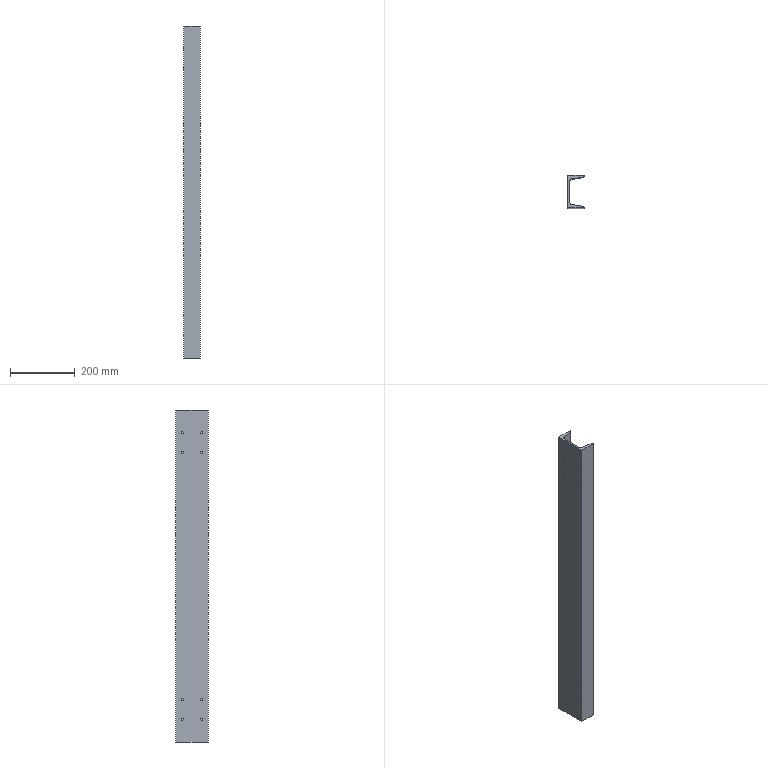Part | SolidWorks | features Extrusion 1, HoleWzd 1 | 1 solid | 30 faces | box 50 x 100 x 1022 mm | volume 1354327 mm3 | cylinder 20 | plane 10 | commonest cylinder face diameters 6.8 x16 9 x2 17 x2
STEP:
#1=CARTESIAN_POINT('',(-44.,-20.,66.6));
#2=VERTEX_POINT('',#1);
#3=CARTESIAN_POINT('',(-44.,-20.,73.4));
#4=VERTEX_POINT('',#3);
#5=CARTESIAN_POINT('',(-44.,-20.,70.));
#6=DIRECTION('',(-1.,0.,0.));
#7=DIRECTION('',(0.,0.,1.));
#8=AXIS2_PLACEMENT_3D('',#5,#6,#7);
#9=CIRCLE('',#8,3.4);
#10=EDGE_CURVE('',#2,#4,#9,.T.);
#11=ORIENTED_EDGE('',*,*,#10,.F.);
#12=CARTESIAN_POINT('',(-50.,-20.,66.6));
#13=VERTEX_POINT('',#12);
#14=CARTESIAN_POINT('',(-50.,-20.,66.6));
#15=DIRECTION('',(-1.,0.,0.));
#16=VECTOR('',#15,1000.);
#17=LINE('',#14,#16);
#18=EDGE_CURVE('',#2,#13,#17,.T.);
#19=ORIENTED_EDGE('',*,*,#18,.T.);
#20=CARTESIAN_POINT('',(-50.,-20.,73.4));
#21=VERTEX_POINT('',#20);
#22=CARTESIAN_POINT('',(-50.,-20.,70.));
#23=DIRECTION('',(-1.,0.,0.));
#24=DIRECTION('',(0.,0.,1.));
#25=AXIS2_PLACEMENT_3D('',#22,#23,#24);
#26=CIRCLE('',#25,3.4);
#27=EDGE_CURVE('',#13,#21,#26,.T.);
#28=ORIENTED_EDGE('',*,*,#27,.T.);
#29=CARTESIAN_POINT('',(-50.,-20.,73.4));
#30=DIRECTION('',(-1.,0.,0.));
#31=VECTOR('',#30,1000.);
#32=LINE('',#29,#31);
#33=EDGE_CURVE('',#4,#21,#32,.T.);
#34=ORIENTED_EDGE('',*,*,#33,.F.);
#35=EDGE_LOOP('',(#11,#19,#28,#34));
#36=FACE_OUTER_BOUND('',#35,.T.);
#37=CARTESIAN_POINT('',(-50.,-20.,70.));
#38=DIRECTION('',(-1.,0.,0.));
#39=DIRECTION('',(0.,0.,1.));
#40=AXIS2_PLACEMENT_3D('',#37,#38,#39);
#41=CYLINDRICAL_SURFACE('',#40,3.4);
#42=ADVANCED_FACE('',(#36),#41,.F.);
#43=CARTESIAN_POINT('',(-44.,-20.,126.6));
#44=VERTEX_POINT('',#43);
#45=CARTESIAN_POINT('',(-44.,-20.,133.4));
#46=VERTEX_POINT('',#45);
#47=CARTESIAN_POINT('',(-44.,-20.,130.));
#48=DIRECTION('',(-1.,0.,0.));
#49=DIRECTION('',(0.,0.,1.));
#50=AXIS2_PLACEMENT_3D('',#47,#48,#49);
#51=CIRCLE('',#50,3.4);
#52=EDGE_CURVE('',#44,#46,#51,.T.);
#53=ORIENTED_EDGE('',*,*,#52,.F.);
#54=CARTESIAN_POINT('',(-50.,-20.,126.6));
#55=VERTEX_POINT('',#54);
#56=CARTESIAN_POINT('',(-50.,-20.,126.6));
#57=DIRECTION('',(-1.,0.,0.));
#58=VECTOR('',#57,1000.);
#59=LINE('',#56,#58);
#60=EDGE_CURVE('',#44,#55,#59,.T.);
#61=ORIENTED_EDGE('',*,*,#60,.T.);
#62=CARTESIAN_POINT('',(-50.,-20.,133.4));
#63=VERTEX_POINT('',#62);
#64=CARTESIAN_POINT('',(-50.,-20.,130.));
#65=DIRECTION('',(-1.,0.,0.));
#66=DIRECTION('',(0.,0.,1.));
#67=AXIS2_PLACEMENT_3D('',#64,#65,#66);
#68=CIRCLE('',#67,3.4);
#69=EDGE_CURVE('',#55,#63,#68,.T.);
#70=ORIENTED_EDGE('',*,*,#69,.T.);
#71=CARTESIAN_POINT('',(-50.,-20.,133.4));
#72=DIRECTION('',(-1.,0.,0.));
#73=VECTOR('',#72,1000.);
#74=LINE('',#71,#73);
#75=EDGE_CURVE('',#46,#63,#74,.T.);
#76=ORIENTED_EDGE('',*,*,#75,.F.);
#77=EDGE_LOOP('',(#53,#61,#70,#76));
#78=FACE_OUTER_BOUND('',#77,.T.);
#79=CARTESIAN_POINT('',(-50.,-20.,130.));
#80=DIRECTION('',(-1.,0.,0.));
#81=DIRECTION('',(0.,0.,1.));
#82=AXIS2_PLACEMENT_3D('',#79,#80,#81);
#83=CYLINDRICAL_SURFACE('',#82,3.4);
#84=ADVANCED_FACE('',(#78),#83,.F.);
#85=CARTESIAN_POINT('',(-44.,-80.,126.6));
#86=VERTEX_POINT('',#85);
#87=CARTESIAN_POINT('',(-44.,-81.441,126.92));
#88=VERTEX_POINT('',#87);
#89=CARTESIAN_POINT('',(-44.,-80.,130.));
#90=DIRECTION('',(-1.,0.,0.));
#91=DIRECTION('',(0.,0.,1.));
#92=AXIS2_PLACEMENT_3D('',#89,#90,#91);
#93=CIRCLE('',#92,3.4);
#94=EDGE_CURVE('',#86,#88,#93,.T.);
#95=ORIENTED_EDGE('',*,*,#94,.F.);
#96=CARTESIAN_POINT('',(-50.,-80.,126.6));
#97=VERTEX_POINT('',#96);
#98=CARTESIAN_POINT('',(-50.,-80.,126.6));
#99=DIRECTION('',(-1.,0.,0.));
#100=VECTOR('',#99,1000.);
#101=LINE('',#98,#100);
#102=EDGE_CURVE('',#86,#97,#101,.T.);
#103=ORIENTED_EDGE('',*,*,#102,.T.);
#104=CARTESIAN_POINT('',(-50.,-80.,133.4));
#105=VERTEX_POINT('',#104);
#106=CARTESIAN_POINT('',(-50.,-80.,130.));
#107=DIRECTION('',(-1.,0.,0.));
#108=DIRECTION('',(0.,0.,1.));
#109=AXIS2_PLACEMENT_3D('',#106,#107,#108);
#110=CIRCLE('',#109,3.4);
#111=EDGE_CURVE('',#97,#105,#110,.T.);
#112=ORIENTED_EDGE('',*,*,#111,.T.);
#113=CARTESIAN_POINT('',(-44.,-80.,133.4));
#114=VERTEX_POINT('',#113);
#115=CARTESIAN_POINT('',(-50.,-80.,133.4));
#116=DIRECTION('',(-1.,0.,0.));
#117=VECTOR('',#116,1000.);
#118=LINE('',#115,#117);
#119=EDGE_CURVE('',#114,#105,#118,.T.);
#120=ORIENTED_EDGE('',*,*,#119,.F.);
#121=CARTESIAN_POINT('',(-44.,-81.441,133.08));
#122=VERTEX_POINT('',#121);
#123=CARTESIAN_POINT('',(-44.,-80.,130.));
#124=DIRECTION('',(-1.,0.,0.));
#125=DIRECTION('',(0.,0.,1.));
#126=AXIS2_PLACEMENT_3D('',#123,#124,#125);
#127=CIRCLE('',#126,3.4);
#128=EDGE_CURVE('',#122,#114,#127,.T.);
#129=ORIENTED_EDGE('',*,*,#128,.F.);
#130=CARTESIAN_POINT('',(-44.,-81.441,126.92));
#131=CARTESIAN_POINT('',(-44.,-81.735,127.058));
#132=CARTESIAN_POINT('',(-43.985,-82.002,127.233));
#133=CARTESIAN_POINT('',(-43.951,-82.365,127.552));
#134=CARTESIAN_POINT('',(-43.937,-82.479,127.667));
#135=CARTESIAN_POINT('',(-43.909,-82.687,127.91));
#136=CARTESIAN_POINT('',(-43.894,-82.782,128.039));
#137=CARTESIAN_POINT('',(-43.865,-82.954,128.308));
#138=CARTESIAN_POINT('',(-43.85,-83.031,128.451));
#139=CARTESIAN_POINT('',(-43.824,-83.163,128.744));
#140=CARTESIAN_POINT('',(-43.812,-83.219,128.894));
#141=CARTESIAN_POINT('',(-43.783,-83.353,129.353));
#142=CARTESIAN_POINT('',(-43.771,-83.4,129.679));
#143=CARTESIAN_POINT('',(-43.771,-83.4,130.159));
#144=CARTESIAN_POINT('',(-43.774,-83.389,130.319));
#145=CARTESIAN_POINT('',(-43.784,-83.344,130.637));
#146=CARTESIAN_POINT('',(-43.792,-83.309,130.796));
#147=CARTESIAN_POINT('',(-43.812,-83.22,131.105));
#148=CARTESIAN_POINT('',(-43.824,-83.164,131.254));
#149=CARTESIAN_POINT('',(-43.85,-83.033,131.546));
#150=CARTESIAN_POINT('',(-43.864,-82.956,131.688));
#151=CARTESIAN_POINT('',(-43.909,-82.697,132.095));
#152=CARTESIAN_POINT('',(-43.939,-82.49,132.338));
#153=CARTESIAN_POINT('',(-43.985,-82.005,132.765));
#154=CARTESIAN_POINT('',(-44.,-81.735,132.942));
#155=CARTESIAN_POINT('',(-44.,-81.441,133.08));
#156=B_SPLINE_CURVE_WITH_KNOTS('',3,(#130,#131,#132,#133,#134,#135,#136,#137,#138,#139,#140,#141,#142,#143,#144,#145,#146,#147,#148,#149,#150,#151,#152,#153,#154,#155),.UNSPECIFIED.,.F.,.F.,(4,2,2,2,2,2,2,2,2,2,2,2,4),(0.,0.0009601,0.00144,0.00192,0.0024,0.00288,0.003841,0.004321,0.004801,0.005281,0.005761,0.006721,0.007681),.UNSPECIFIED.);
#157=EDGE_CURVE('',#88,#122,#156,.T.);
#158=ORIENTED_EDGE('',*,*,#157,.F.);
#159=EDGE_LOOP('',(#95,#103,#112,#120,#129,#158));
#160=FACE_OUTER_BOUND('',#159,.T.);
#161=CARTESIAN_POINT('',(-50.,-80.,130.));
#162=DIRECTION('',(-1.,0.,0.));
#163=DIRECTION('',(0.,0.,1.));
#164=AXIS2_PLACEMENT_3D('',#161,#162,#163);
#165=CYLINDRICAL_SURFACE('',#164,3.4);
#166=ADVANCED_FACE('',(#160),#165,.F.);
#167=CARTESIAN_POINT('',(-44.,-80.,66.6));
#168=VERTEX_POINT('',#167);
#169=CARTESIAN_POINT('',(-44.,-81.441,66.92));
#170=VERTEX_POINT('',#169);
#171=CARTESIAN_POINT('',(-44.,-80.,70.));
#172=DIRECTION('',(-1.,0.,0.));
#173=DIRECTION('',(0.,0.,1.));
#174=AXIS2_PLACEMENT_3D('',#171,#172,#173);
#175=CIRCLE('',#174,3.4);
#176=EDGE_CURVE('',#168,#170,#175,.T.);
#177=ORIENTED_EDGE('',*,*,#176,.F.);
#178=CARTESIAN_POINT('',(-50.,-80.,66.6));
#179=VERTEX_POINT('',#178);
#180=CARTESIAN_POINT('',(-50.,-80.,66.6));
#181=DIRECTION('',(-1.,0.,0.));
#182=VECTOR('',#181,1000.);
#183=LINE('',#180,#182);
#184=EDGE_CURVE('',#168,#179,#183,.T.);
#185=ORIENTED_EDGE('',*,*,#184,.T.);
#186=CARTESIAN_POINT('',(-50.,-80.,73.4));
#187=VERTEX_POINT('',#186);
#188=CARTESIAN_POINT('',(-50.,-80.,70.));
#189=DIRECTION('',(-1.,0.,0.));
#190=DIRECTION('',(0.,0.,1.));
#191=AXIS2_PLACEMENT_3D('',#188,#189,#190);
#192=CIRCLE('',#191,3.4);
#193=EDGE_CURVE('',#179,#187,#192,.T.);
#194=ORIENTED_EDGE('',*,*,#193,.T.);
#195=CARTESIAN_POINT('',(-44.,-80.,73.4));
#196=VERTEX_POINT('',#195);
#197=CARTESIAN_POINT('',(-50.,-80.,73.4));
#198=DIRECTION('',(-1.,0.,0.));
#199=VECTOR('',#198,1000.);
#200=LINE('',#197,#199);
#201=EDGE_CURVE('',#196,#187,#200,.T.);
#202=ORIENTED_EDGE('',*,*,#201,.F.);
#203=CARTESIAN_POINT('',(-44.,-81.441,73.08));
#204=VERTEX_POINT('',#203);
#205=CARTESIAN_POINT('',(-44.,-80.,70.));
#206=DIRECTION('',(-1.,0.,0.));
#207=DIRECTION('',(0.,0.,1.));
#208=AXIS2_PLACEMENT_3D('',#205,#206,#207);
#209=CIRCLE('',#208,3.4);
#210=EDGE_CURVE('',#204,#196,#209,.T.);
#211=ORIENTED_EDGE('',*,*,#210,.F.);
#212=CARTESIAN_POINT('',(-44.,-81.441,66.92));
#213=CARTESIAN_POINT('',(-44.,-81.735,67.058));
#214=CARTESIAN_POINT('',(-43.985,-82.002,67.233));
#215=CARTESIAN_POINT('',(-43.951,-82.365,67.552));
#216=CARTESIAN_POINT('',(-43.937,-82.479,67.667));
#217=CARTESIAN_POINT('',(-43.909,-82.687,67.91));
#218=CARTESIAN_POINT('',(-43.894,-82.782,68.039));
#219=CARTESIAN_POINT('',(-43.865,-82.954,68.308));
#220=CARTESIAN_POINT('',(-43.85,-83.031,68.451));
#221=CARTESIAN_POINT('',(-43.824,-83.163,68.744));
#222=CARTESIAN_POINT('',(-43.812,-83.219,68.894));
#223=CARTESIAN_POINT('',(-43.783,-83.353,69.353));
#224=CARTESIAN_POINT('',(-43.771,-83.4,69.679));
#225=CARTESIAN_POINT('',(-43.771,-83.4,70.159));
#226=CARTESIAN_POINT('',(-43.774,-83.389,70.319));
#227=CARTESIAN_POINT('',(-43.784,-83.344,70.637));
#228=CARTESIAN_POINT('',(-43.792,-83.309,70.796));
#229=CARTESIAN_POINT('',(-43.812,-83.22,71.105));
#230=CARTESIAN_POINT('',(-43.824,-83.164,71.254));
#231=CARTESIAN_POINT('',(-43.85,-83.033,71.546));
#232=CARTESIAN_POINT('',(-43.864,-82.956,71.688));
#233=CARTESIAN_POINT('',(-43.909,-82.697,72.095));
#234=CARTESIAN_POINT('',(-43.939,-82.49,72.338));
#235=CARTESIAN_POINT('',(-43.985,-82.005,72.765));
#236=CARTESIAN_POINT('',(-44.,-81.735,72.942));
#237=CARTESIAN_POINT('',(-44.,-81.441,73.08));
#238=B_SPLINE_CURVE_WITH_KNOTS('',3,(#212,#213,#214,#215,#216,#217,#218,#219,#220,#221,#222,#223,#224,#225,#226,#227,#228,#229,#230,#231,#232,#233,#234,#235,#236,#237),.UNSPECIFIED.,.F.,.F.,(4,2,2,2,2,2,2,2,2,2,2,2,4),(0.,0.0009601,0.00144,0.00192,0.0024,0.00288,0.003841,0.004321,0.004801,0.005281,0.005761,0.006721,0.007681),.UNSPECIFIED.);
#239=EDGE_CURVE('',#170,#204,#238,.T.);
#240=ORIENTED_EDGE('',*,*,#239,.F.);
#241=EDGE_LOOP('',(#177,#185,#194,#202,#211,#240));
#242=FACE_OUTER_BOUND('',#241,.T.);
#243=CARTESIAN_POINT('',(-50.,-80.,70.));
#244=DIRECTION('',(-1.,0.,0.));
#245=DIRECTION('',(0.,0.,1.));
#246=AXIS2_PLACEMENT_3D('',#243,#244,#245);
#247=CYLINDRICAL_SURFACE('',#246,3.4);
#248=ADVANCED_FACE('',(#242),#247,.F.);
#249=CARTESIAN_POINT('',(-44.,-20.,888.6));
#250=VERTEX_POINT('',#249);
#251=CARTESIAN_POINT('',(-44.,-20.,895.4));
#252=VERTEX_POINT('',#251);
#253=CARTESIAN_POINT('',(-44.,-20.,892.));
#254=DIRECTION('',(-1.,0.,0.));
#255=DIRECTION('',(0.,0.,1.));
#256=AXIS2_PLACEMENT_3D('',#253,#254,#255);
#257=CIRCLE('',#256,3.4);
#258=EDGE_CURVE('',#250,#252,#257,.T.);
#259=ORIENTED_EDGE('',*,*,#258,.F.);
#260=CARTESIAN_POINT('',(-50.,-20.,888.6));
#261=VERTEX_POINT('',#260);
#262=CARTESIAN_POINT('',(-50.,-20.,888.6));
#263=DIRECTION('',(-1.,0.,0.));
#264=VECTOR('',#263,1000.);
#265=LINE('',#262,#264);
#266=EDGE_CURVE('',#250,#261,#265,.T.);
#267=ORIENTED_EDGE('',*,*,#266,.T.);
#268=CARTESIAN_POINT('',(-50.,-20.,895.4));
#269=VERTEX_POINT('',#268);
#270=CARTESIAN_POINT('',(-50.,-20.,892.));
#271=DIRECTION('',(-1.,0.,0.));
#272=DIRECTION('',(0.,0.,1.));
#273=AXIS2_PLACEMENT_3D('',#270,#271,#272);
#274=CIRCLE('',#273,3.4);
#275=EDGE_CURVE('',#261,#269,#274,.T.);
#276=ORIENTED_EDGE('',*,*,#275,.T.);
#277=CARTESIAN_POINT('',(-50.,-20.,895.4));
#278=DIRECTION('',(-1.,0.,0.));
#279=VECTOR('',#278,1000.);
#280=LINE('',#277,#279);
#281=EDGE_CURVE('',#252,#269,#280,.T.);
#282=ORIENTED_EDGE('',*,*,#281,.F.);
#283=EDGE_LOOP('',(#259,#267,#276,#282));
#284=FACE_OUTER_BOUND('',#283,.T.);
#285=CARTESIAN_POINT('',(-50.,-20.,892.));
#286=DIRECTION('',(-1.,0.,0.));
#287=DIRECTION('',(0.,0.,1.));
#288=AXIS2_PLACEMENT_3D('',#285,#286,#287);
#289=CYLINDRICAL_SURFACE('',#288,3.4);
#290=ADVANCED_FACE('',(#284),#289,.F.);
#291=CARTESIAN_POINT('',(-44.,-20.,948.6));
#292=VERTEX_POINT('',#291);
#293=CARTESIAN_POINT('',(-44.,-20.,955.4));
#294=VERTEX_POINT('',#293);
#295=CARTESIAN_POINT('',(-44.,-20.,952.));
#296=DIRECTION('',(-1.,0.,0.));
#297=DIRECTION('',(0.,0.,1.));
#298=AXIS2_PLACEMENT_3D('',#295,#296,#297);
#299=CIRCLE('',#298,3.4);
#300=EDGE_CURVE('',#292,#294,#299,.T.);
#301=ORIENTED_EDGE('',*,*,#300,.F.);
#302=CARTESIAN_POINT('',(-50.,-20.,948.6));
#303=VERTEX_POINT('',#302);
#304=CARTESIAN_POINT('',(-50.,-20.,948.6));
#305=DIRECTION('',(-1.,0.,0.));
#306=VECTOR('',#305,1000.);
#307=LINE('',#304,#306);
#308=EDGE_CURVE('',#292,#303,#307,.T.);
#309=ORIENTED_EDGE('',*,*,#308,.T.);
#310=CARTESIAN_POINT('',(-50.,-20.,955.4));
#311=VERTEX_POINT('',#310);
#312=CARTESIAN_POINT('',(-50.,-20.,952.));
#313=DIRECTION('',(-1.,0.,0.));
#314=DIRECTION('',(0.,0.,1.));
#315=AXIS2_PLACEMENT_3D('',#312,#313,#314);
#316=CIRCLE('',#315,3.4);
#317=EDGE_CURVE('',#303,#311,#316,.T.);
#318=ORIENTED_EDGE('',*,*,#317,.T.);
#319=CARTESIAN_POINT('',(-50.,-20.,955.4));
#320=DIRECTION('',(-1.,0.,0.));
#321=VECTOR('',#320,1000.);
#322=LINE('',#319,#321);
#323=EDGE_CURVE('',#294,#311,#322,.T.);
#324=ORIENTED_EDGE('',*,*,#323,.F.);
#325=EDGE_LOOP('',(#301,#309,#318,#324));
#326=FACE_OUTER_BOUND('',#325,.T.);
#327=CARTESIAN_POINT('',(-50.,-20.,952.));
#328=DIRECTION('',(-1.,0.,0.));
#329=DIRECTION('',(0.,0.,1.));
#330=AXIS2_PLACEMENT_3D('',#327,#328,#329);
#331=CYLINDRICAL_SURFACE('',#330,3.4);
#332=ADVANCED_FACE('',(#326),#331,.F.);
#333=CARTESIAN_POINT('',(-44.,-80.,948.6));
#334=VERTEX_POINT('',#333);
#335=CARTESIAN_POINT('',(-44.,-81.441,948.92));
#336=VERTEX_POINT('',#335);
#337=CARTESIAN_POINT('',(-44.,-80.,952.));
#338=DIRECTION('',(-1.,0.,0.));
#339=DIRECTION('',(0.,0.,1.));
#340=AXIS2_PLACEMENT_3D('',#337,#338,#339);
#341=CIRCLE('',#340,3.4);
#342=EDGE_CURVE('',#334,#336,#341,.T.);
#343=ORIENTED_EDGE('',*,*,#342,.F.);
#344=CARTESIAN_POINT('',(-50.,-80.,948.6));
#345=VERTEX_POINT('',#344);
#346=CARTESIAN_POINT('',(-50.,-80.,948.6));
#347=DIRECTION('',(-1.,0.,0.));
#348=VECTOR('',#347,1000.);
#349=LINE('',#346,#348);
#350=EDGE_CURVE('',#334,#345,#349,.T.);
#351=ORIENTED_EDGE('',*,*,#350,.T.);
#352=CARTESIAN_POINT('',(-50.,-80.,955.4));
#353=VERTEX_POINT('',#352);
#354=CARTESIAN_POINT('',(-50.,-80.,952.));
#355=DIRECTION('',(-1.,0.,0.));
#356=DIRECTION('',(0.,0.,1.));
#357=AXIS2_PLACEMENT_3D('',#354,#355,#356);
#358=CIRCLE('',#357,3.4);
#359=EDGE_CURVE('',#345,#353,#358,.T.);
#360=ORIENTED_EDGE('',*,*,#359,.T.);
#361=CARTESIAN_POINT('',(-44.,-80.,955.4));
#362=VERTEX_POINT('',#361);
#363=CARTESIAN_POINT('',(-50.,-80.,955.4));
#364=DIRECTION('',(-1.,0.,0.));
#365=VECTOR('',#364,1000.);
#366=LINE('',#363,#365);
#367=EDGE_CURVE('',#362,#353,#366,.T.);
#368=ORIENTED_EDGE('',*,*,#367,.F.);
#369=CARTESIAN_POINT('',(-44.,-81.441,955.08));
#370=VERTEX_POINT('',#369);
#371=CARTESIAN_POINT('',(-44.,-80.,952.));
#372=DIRECTION('',(-1.,0.,0.));
#373=DIRECTION('',(0.,0.,1.));
#374=AXIS2_PLACEMENT_3D('',#371,#372,#373);
#375=CIRCLE('',#374,3.4);
#376=EDGE_CURVE('',#370,#362,#375,.T.);
#377=ORIENTED_EDGE('',*,*,#376,.F.);
#378=CARTESIAN_POINT('',(-44.,-81.441,948.92));
#379=CARTESIAN_POINT('',(-44.,-81.735,949.058));
#380=CARTESIAN_POINT('',(-43.985,-82.002,949.233));
#381=CARTESIAN_POINT('',(-43.951,-82.365,949.552));
#382=CARTESIAN_POINT('',(-43.937,-82.479,949.667));
#383=CARTESIAN_POINT('',(-43.909,-82.687,949.91));
#384=CARTESIAN_POINT('',(-43.894,-82.782,950.039));
#385=CARTESIAN_POINT('',(-43.865,-82.954,950.308));
#386=CARTESIAN_POINT('',(-43.85,-83.031,950.451));
#387=CARTESIAN_POINT('',(-43.824,-83.163,950.744));
#388=CARTESIAN_POINT('',(-43.812,-83.219,950.894));
#389=CARTESIAN_POINT('',(-43.783,-83.353,951.353));
#390=CARTESIAN_POINT('',(-43.771,-83.4,951.679));
#391=CARTESIAN_POINT('',(-43.771,-83.4,952.159));
#392=CARTESIAN_POINT('',(-43.774,-83.389,952.319));
#393=CARTESIAN_POINT('',(-43.784,-83.344,952.637));
#394=CARTESIAN_POINT('',(-43.792,-83.309,952.796));
#395=CARTESIAN_POINT('',(-43.812,-83.22,953.105));
#396=CARTESIAN_POINT('',(-43.824,-83.164,953.254));
#397=CARTESIAN_POINT('',(-43.85,-83.033,953.546));
#398=CARTESIAN_POINT('',(-43.864,-82.956,953.688));
#399=CARTESIAN_POINT('',(-43.909,-82.697,954.095));
#400=CARTESIAN_POINT('',(-43.939,-82.49,954.338));
#401=CARTESIAN_POINT('',(-43.985,-82.005,954.765));
#402=CARTESIAN_POINT('',(-44.,-81.735,954.942));
#403=CARTESIAN_POINT('',(-44.,-81.441,955.08));
#404=B_SPLINE_CURVE_WITH_KNOTS('',3,(#378,#379,#380,#381,#382,#383,#384,#385,#386,#387,#388,#389,#390,#391,#392,#393,#394,#395,#396,#397,#398,#399,#400,#401,#402,#403),.UNSPECIFIED.,.F.,.F.,(4,2,2,2,2,2,2,2,2,2,2,2,4),(0.,0.0009601,0.00144,0.00192,0.0024,0.00288,0.003841,0.004321,0.004801,0.005281,0.005761,0.006721,0.007681),.UNSPECIFIED.);
#405=EDGE_CURVE('',#336,#370,#404,.T.);
#406=ORIENTED_EDGE('',*,*,#405,.F.);
#407=EDGE_LOOP('',(#343,#351,#360,#368,#377,#406));
#408=FACE_OUTER_BOUND('',#407,.T.);
#409=CARTESIAN_POINT('',(-50.,-80.,952.));
#410=DIRECTION('',(-1.,0.,0.));
#411=DIRECTION('',(0.,0.,1.));
#412=AXIS2_PLACEMENT_3D('',#409,#410,#411);
#413=CYLINDRICAL_SURFACE('',#412,3.4);
#414=ADVANCED_FACE('',(#408),#413,.F.);
#415=CARTESIAN_POINT('',(-44.,-80.,888.6));
#416=VERTEX_POINT('',#415);
#417=CARTESIAN_POINT('',(-44.,-81.441,888.92));
#418=VERTEX_POINT('',#417);
#419=CARTESIAN_POINT('',(-44.,-80.,892.));
#420=DIRECTION('',(-1.,0.,0.));
#421=DIRECTION('',(0.,0.,1.));
#422=AXIS2_PLACEMENT_3D('',#419,#420,#421);
#423=CIRCLE('',#422,3.4);
#424=EDGE_CURVE('',#416,#418,#423,.T.);
#425=ORIENTED_EDGE('',*,*,#424,.F.);
#426=CARTESIAN_POINT('',(-50.,-80.,888.6));
#427=VERTEX_POINT('',#426);
#428=CARTESIAN_POINT('',(-50.,-80.,888.6));
#429=DIRECTION('',(-1.,0.,0.));
#430=VECTOR('',#429,1000.);
#431=LINE('',#428,#430);
#432=EDGE_CURVE('',#416,#427,#431,.T.);
#433=ORIENTED_EDGE('',*,*,#432,.T.);
#434=CARTESIAN_POINT('',(-50.,-80.,895.4));
#435=VERTEX_POINT('',#434);
#436=CARTESIAN_POINT('',(-50.,-80.,892.));
#437=DIRECTION('',(-1.,0.,0.));
#438=DIRECTION('',(0.,0.,1.));
#439=AXIS2_PLACEMENT_3D('',#436,#437,#438);
#440=CIRCLE('',#439,3.4);
#441=EDGE_CURVE('',#427,#435,#440,.T.);
#442=ORIENTED_EDGE('',*,*,#441,.T.);
#443=CARTESIAN_POINT('',(-44.,-80.,895.4));
#444=VERTEX_POINT('',#443);
#445=CARTESIAN_POINT('',(-50.,-80.,895.4));
#446=DIRECTION('',(-1.,0.,0.));
#447=VECTOR('',#446,1000.);
#448=LINE('',#445,#447);
#449=EDGE_CURVE('',#444,#435,#448,.T.);
#450=ORIENTED_EDGE('',*,*,#449,.F.);
#451=CARTESIAN_POINT('',(-44.,-81.441,895.08));
#452=VERTEX_POINT('',#451);
#453=CARTESIAN_POINT('',(-44.,-80.,892.));
#454=DIRECTION('',(-1.,0.,0.));
#455=DIRECTION('',(0.,0.,1.));
#456=AXIS2_PLACEMENT_3D('',#453,#454,#455);
#457=CIRCLE('',#456,3.4);
#458=EDGE_CURVE('',#452,#444,#457,.T.);
#459=ORIENTED_EDGE('',*,*,#458,.F.);
#460=CARTESIAN_POINT('',(-44.,-81.441,888.92));
#461=CARTESIAN_POINT('',(-44.,-81.735,889.058));
#462=CARTESIAN_POINT('',(-43.985,-82.002,889.233));
#463=CARTESIAN_POINT('',(-43.951,-82.365,889.552));
#464=CARTESIAN_POINT('',(-43.937,-82.479,889.667));
#465=CARTESIAN_POINT('',(-43.909,-82.687,889.91));
#466=CARTESIAN_POINT('',(-43.894,-82.782,890.039));
#467=CARTESIAN_POINT('',(-43.865,-82.954,890.308));
#468=CARTESIAN_POINT('',(-43.85,-83.031,890.451));
#469=CARTESIAN_POINT('',(-43.824,-83.163,890.744));
#470=CARTESIAN_POINT('',(-43.812,-83.219,890.894));
#471=CARTESIAN_POINT('',(-43.783,-83.353,891.353));
#472=CARTESIAN_POINT('',(-43.771,-83.4,891.679));
#473=CARTESIAN_POINT('',(-43.771,-83.4,892.159));
#474=CARTESIAN_POINT('',(-43.774,-83.389,892.319));
#475=CARTESIAN_POINT('',(-43.784,-83.344,892.637));
#476=CARTESIAN_POINT('',(-43.792,-83.309,892.796));
#477=CARTESIAN_POINT('',(-43.812,-83.22,893.105));
#478=CARTESIAN_POINT('',(-43.824,-83.164,893.254));
#479=CARTESIAN_POINT('',(-43.85,-83.033,893.546));
#480=CARTESIAN_POINT('',(-43.864,-82.956,893.688));
#481=CARTESIAN_POINT('',(-43.909,-82.697,894.095));
#482=CARTESIAN_POINT('',(-43.939,-82.49,894.338));
#483=CARTESIAN_POINT('',(-43.985,-82.005,894.765));
#484=CARTESIAN_POINT('',(-44.,-81.735,894.942));
#485=CARTESIAN_POINT('',(-44.,-81.441,895.08));
#486=B_SPLINE_CURVE_WITH_KNOTS('',3,(#460,#461,#462,#463,#464,#465,#466,#467,#468,#469,#470,#471,#472,#473,#474,#475,#476,#477,#478,#479,#480,#481,#482,#483,#484,#485),.UNSPECIFIED.,.F.,.F.,(4,2,2,2,2,2,2,2,2,2,2,2,4),(0.,0.0009601,0.00144,0.00192,0.0024,0.00288,0.003841,0.004321,0.004801,0.005281,0.005761,0.006721,0.007681),.UNSPECIFIED.);
#487=EDGE_CURVE('',#418,#452,#486,.T.);
#488=ORIENTED_EDGE('',*,*,#487,.F.);
#489=EDGE_LOOP('',(#425,#433,#442,#450,#459,#488));
#490=FACE_OUTER_BOUND('',#489,.T.);
#491=CARTESIAN_POINT('',(-50.,-80.,892.));
#492=DIRECTION('',(-1.,0.,0.));
#493=DIRECTION('',(0.,0.,1.));
#494=AXIS2_PLACEMENT_3D('',#491,#492,#493);
#495=CYLINDRICAL_SURFACE('',#494,3.4);
#496=ADVANCED_FACE('',(#490),#495,.F.);
#497=CARTESIAN_POINT('',(0.,-1.075,0.));
#498=VERTEX_POINT('',#497);
#499=CARTESIAN_POINT('',(0.,0.,0.));
#500=VERTEX_POINT('',#499);
#501=CARTESIAN_POINT('',(0.,-1.075,0.));
#502=DIRECTION('',(0.,1.,0.));
#503=VECTOR('',#502,1000.);
#504=LINE('',#501,#503);
#505=EDGE_CURVE('',#498,#500,#504,.T.);
#506=ORIENTED_EDGE('',*,*,#505,.T.);
#507=CARTESIAN_POINT('',(0.,0.,1022.));
#508=VERTEX_POINT('',#507);
#509=CARTESIAN_POINT('',(0.,0.,1022.));
#510=DIRECTION('',(0.,0.,-1.));
#511=VECTOR('',#510,1000.);
#512=LINE('',#509,#511);
#513=EDGE_CURVE('',#508,#500,#512,.T.);
#514=ORIENTED_EDGE('',*,*,#513,.F.);
#515=CARTESIAN_POINT('',(0.,-1.075,1022.));
#516=VERTEX_POINT('',#515);
#517=CARTESIAN_POINT('',(0.,-1.075,1022.));
#518=DIRECTION('',(0.,1.,0.));
#519=VECTOR('',#518,1000.);
#520=LINE('',#517,#519);
#521=EDGE_CURVE('',#516,#508,#520,.T.);
#522=ORIENTED_EDGE('',*,*,#521,.F.);
#523=CARTESIAN_POINT('',(0.,-1.075,1022.));
#524=DIRECTION('',(0.,0.,-1.));
#525=VECTOR('',#524,1000.);
#526=LINE('',#523,#525);
#527=EDGE_CURVE('',#516,#498,#526,.T.);
#528=ORIENTED_EDGE('',*,*,#527,.T.);
#529=EDGE_LOOP('',(#506,#514,#522,#528));
#530=FACE_OUTER_BOUND('',#529,.T.);
#531=CARTESIAN_POINT('',(0.,-1.075,1022.));
#532=DIRECTION('',(-1.,0.,0.));
#533=DIRECTION('',(0.,0.,1.));
#534=AXIS2_PLACEMENT_3D('',#531,#532,#533);
#535=PLANE('',#534);
#536=ADVANCED_FACE('',(#530),#535,.F.);
#537=CARTESIAN_POINT('',(-50.,0.,0.));
#538=VERTEX_POINT('',#537);
#539=CARTESIAN_POINT('',(0.,0.,0.));
#540=DIRECTION('',(-1.,0.,0.));
#541=VECTOR('',#540,1000.);
#542=LINE('',#539,#541);
#543=EDGE_CURVE('',#500,#538,#542,.T.);
#544=ORIENTED_EDGE('',*,*,#543,.T.);
#545=CARTESIAN_POINT('',(-50.,0.,1022.));
#546=VERTEX_POINT('',#545);
#547=CARTESIAN_POINT('',(-50.,0.,1022.));
#548=DIRECTION('',(0.,0.,-1.));
#549=VECTOR('',#548,1000.);
#550=LINE('',#547,#549);
#551=EDGE_CURVE('',#546,#538,#550,.T.);
#552=ORIENTED_EDGE('',*,*,#551,.F.);
#553=CARTESIAN_POINT('',(0.,0.,1022.));
#554=DIRECTION('',(-1.,0.,0.));
#555=VECTOR('',#554,1000.);
#556=LINE('',#553,#555);
#557=EDGE_CURVE('',#508,#546,#556,.T.);
#558=ORIENTED_EDGE('',*,*,#557,.F.);
#559=ORIENTED_EDGE('',*,*,#513,.T.);
#560=EDGE_LOOP('',(#544,#552,#558,#559));
#561=FACE_OUTER_BOUND('',#560,.T.);
#562=CARTESIAN_POINT('',(0.,0.,1022.));
#563=DIRECTION('',(0.,-1.,0.));
#564=DIRECTION('',(1.,0.,0.));
#565=AXIS2_PLACEMENT_3D('',#562,#563,#564);
#566=PLANE('',#565);
#567=ADVANCED_FACE('',(#561),#566,.F.);
#568=CARTESIAN_POINT('',(-50.,-20.,70.));
#569=DIRECTION('',(-1.,0.,0.));
#570=DIRECTION('',(0.,0.,1.));
#571=AXIS2_PLACEMENT_3D('',#568,#569,#570);
#572=CIRCLE('',#571,3.4);
#573=EDGE_CURVE('',#21,#13,#572,.T.);
#574=ORIENTED_EDGE('',*,*,#573,.F.);
#575=ORIENTED_EDGE('',*,*,#27,.F.);
#576=EDGE_LOOP('',(#574,#575));
#577=FACE_BOUND('',#576,.T.);
#578=CARTESIAN_POINT('',(-50.,-20.,130.));
#579=DIRECTION('',(-1.,0.,0.));
#580=DIRECTION('',(0.,0.,1.));
#581=AXIS2_PLACEMENT_3D('',#578,#579,#580);
#582=CIRCLE('',#581,3.4);
#583=EDGE_CURVE('',#63,#55,#582,.T.);
#584=ORIENTED_EDGE('',*,*,#583,.F.);
#585=ORIENTED_EDGE('',*,*,#69,.F.);
#586=EDGE_LOOP('',(#584,#585));
#587=FACE_BOUND('',#586,.T.);
#588=CARTESIAN_POINT('',(-50.,-80.,130.));
#589=DIRECTION('',(-1.,0.,0.));
#590=DIRECTION('',(0.,0.,1.));
#591=AXIS2_PLACEMENT_3D('',#588,#589,#590);
#592=CIRCLE('',#591,3.4);
#593=EDGE_CURVE('',#105,#97,#592,.T.);
#594=ORIENTED_EDGE('',*,*,#593,.F.);
#595=ORIENTED_EDGE('',*,*,#111,.F.);
#596=EDGE_LOOP('',(#594,#595));
#597=FACE_BOUND('',#596,.T.);
#598=CARTESIAN_POINT('',(-50.,-80.,70.));
#599=DIRECTION('',(-1.,0.,0.));
#600=DIRECTION('',(0.,0.,1.));
#601=AXIS2_PLACEMENT_3D('',#598,#599,#600);
#602=CIRCLE('',#601,3.4);
#603=EDGE_CURVE('',#187,#179,#602,.T.);
#604=ORIENTED_EDGE('',*,*,#603,.F.);
#605=ORIENTED_EDGE('',*,*,#193,.F.);
#606=EDGE_LOOP('',(#604,#605));
#607=FACE_BOUND('',#606,.T.);
#608=CARTESIAN_POINT('',(-50.,-20.,892.));
#609=DIRECTION('',(-1.,0.,0.));
#610=DIRECTION('',(0.,0.,1.));
#611=AXIS2_PLACEMENT_3D('',#608,#609,#610);
#612=CIRCLE('',#611,3.4);
#613=EDGE_CURVE('',#269,#261,#612,.T.);
#614=ORIENTED_EDGE('',*,*,#613,.F.);
#615=ORIENTED_EDGE('',*,*,#275,.F.);
#616=EDGE_LOOP('',(#614,#615));
#617=FACE_BOUND('',#616,.T.);
#618=CARTESIAN_POINT('',(-50.,-20.,952.));
#619=DIRECTION('',(-1.,0.,0.));
#620=DIRECTION('',(0.,0.,1.));
#621=AXIS2_PLACEMENT_3D('',#618,#619,#620);
#622=CIRCLE('',#621,3.4);
#623=EDGE_CURVE('',#311,#303,#622,.T.);
#624=ORIENTED_EDGE('',*,*,#623,.F.);
#625=ORIENTED_EDGE('',*,*,#317,.F.);
#626=EDGE_LOOP('',(#624,#625));
#627=FACE_BOUND('',#626,.T.);
#628=CARTESIAN_POINT('',(-50.,-80.,952.));
#629=DIRECTION('',(-1.,0.,0.));
#630=DIRECTION('',(0.,0.,1.));
#631=AXIS2_PLACEMENT_3D('',#628,#629,#630);
#632=CIRCLE('',#631,3.4);
#633=EDGE_CURVE('',#353,#345,#632,.T.);
#634=ORIENTED_EDGE('',*,*,#633,.F.);
#635=ORIENTED_EDGE('',*,*,#359,.F.);
#636=EDGE_LOOP('',(#634,#635));
#637=FACE_BOUND('',#636,.T.);
#638=CARTESIAN_POINT('',(-50.,-80.,892.));
#639=DIRECTION('',(-1.,0.,0.));
#640=DIRECTION('',(0.,0.,1.));
#641=AXIS2_PLACEMENT_3D('',#638,#639,#640);
#642=CIRCLE('',#641,3.4);
#643=EDGE_CURVE('',#435,#427,#642,.T.);
#644=ORIENTED_EDGE('',*,*,#643,.F.);
#645=ORIENTED_EDGE('',*,*,#441,.F.);
#646=EDGE_LOOP('',(#644,#645));
#647=FACE_BOUND('',#646,.T.);
#648=CARTESIAN_POINT('',(-50.,-100.,0.));
#649=VERTEX_POINT('',#648);
#650=CARTESIAN_POINT('',(-50.,0.,0.));
#651=DIRECTION('',(0.,-1.,0.));
#652=VECTOR('',#651,1000.);
#653=LINE('',#650,#652);
#654=EDGE_CURVE('',#538,#649,#653,.T.);
#655=ORIENTED_EDGE('',*,*,#654,.T.);
#656=CARTESIAN_POINT('',(-50.,-100.,1022.));
#657=VERTEX_POINT('',#656);
#658=CARTESIAN_POINT('',(-50.,-100.,1022.));
#659=DIRECTION('',(0.,0.,-1.));
#660=VECTOR('',#659,1000.);
#661=LINE('',#658,#660);
#662=EDGE_CURVE('',#657,#649,#661,.T.);
#663=ORIENTED_EDGE('',*,*,#662,.F.);
#664=CARTESIAN_POINT('',(-50.,0.,1022.));
#665=DIRECTION('',(0.,-1.,0.));
#666=VECTOR('',#665,1000.);
#667=LINE('',#664,#666);
#668=EDGE_CURVE('',#546,#657,#667,.T.);
#669=ORIENTED_EDGE('',*,*,#668,.F.);
#670=ORIENTED_EDGE('',*,*,#551,.T.);
#671=EDGE_LOOP('',(#655,#663,#669,#670));
#672=FACE_OUTER_BOUND('',#671,.T.);
#673=CARTESIAN_POINT('',(-50.,0.,1022.));
#674=DIRECTION('',(1.,0.,0.));
#675=DIRECTION('',(0.,1.,0.));
#676=AXIS2_PLACEMENT_3D('',#673,#674,#675);
#677=PLANE('',#676);
#678=ADVANCED_FACE('',(#577,#587,#597,#607,#617,#627,#637,#647,#672),#677,.F.);
#679=CARTESIAN_POINT('',(0.,-100.,0.));
#680=VERTEX_POINT('',#679);
#681=CARTESIAN_POINT('',(-50.,-100.,0.));
#682=DIRECTION('',(1.,0.,0.));
#683=VECTOR('',#682,1000.);
#684=LINE('',#681,#683);
#685=EDGE_CURVE('',#649,#680,#684,.T.);
#686=ORIENTED_EDGE('',*,*,#685,.T.);
#687=CARTESIAN_POINT('',(0.,-100.,1022.));
#688=VERTEX_POINT('',#687);
#689=CARTESIAN_POINT('',(0.,-100.,1022.));
#690=DIRECTION('',(0.,0.,-1.));
#691=VECTOR('',#690,1000.);
#692=LINE('',#689,#691);
#693=EDGE_CURVE('',#688,#680,#692,.T.);
#694=ORIENTED_EDGE('',*,*,#693,.F.);
#695=CARTESIAN_POINT('',(-50.,-100.,1022.));
#696=DIRECTION('',(1.,0.,0.));
#697=VECTOR('',#696,1000.);
#698=LINE('',#695,#697);
#699=EDGE_CURVE('',#657,#688,#698,.T.);
#700=ORIENTED_EDGE('',*,*,#699,.F.);
#701=ORIENTED_EDGE('',*,*,#662,.T.);
#702=EDGE_LOOP('',(#686,#694,#700,#701));
#703=FACE_OUTER_BOUND('',#702,.T.);
#704=CARTESIAN_POINT('',(-50.,-100.,1022.));
#705=DIRECTION('',(0.,1.,0.));
#706=DIRECTION('',(0.,0.,1.));
#707=AXIS2_PLACEMENT_3D('',#704,#705,#706);
#708=PLANE('',#707);
#709=ADVANCED_FACE('',(#703),#708,.F.);
#710=CARTESIAN_POINT('',(0.,-98.925,0.));
#711=VERTEX_POINT('',#710);
#712=CARTESIAN_POINT('',(0.,-100.,0.));
#713=DIRECTION('',(0.,1.,0.));
#714=VECTOR('',#713,1000.);
#715=LINE('',#712,#714);
#716=EDGE_CURVE('',#680,#711,#715,.T.);
#717=ORIENTED_EDGE('',*,*,#716,.T.);
#718=CARTESIAN_POINT('',(0.,-98.925,1022.));
#719=VERTEX_POINT('',#718);
#720=CARTESIAN_POINT('',(0.,-98.925,1022.));
#721=DIRECTION('',(0.,0.,-1.));
#722=VECTOR('',#721,1000.);
#723=LINE('',#720,#722);
#724=EDGE_CURVE('',#719,#711,#723,.T.);
#725=ORIENTED_EDGE('',*,*,#724,.F.);
#726=CARTESIAN_POINT('',(0.,-100.,1022.));
#727=DIRECTION('',(0.,1.,0.));
#728=VECTOR('',#727,1000.);
#729=LINE('',#726,#728);
#730=EDGE_CURVE('',#688,#719,#729,.T.);
#731=ORIENTED_EDGE('',*,*,#730,.F.);
#732=ORIENTED_EDGE('',*,*,#693,.T.);
#733=EDGE_LOOP('',(#717,#725,#731,#732));
#734=FACE_OUTER_BOUND('',#733,.T.);
#735=CARTESIAN_POINT('',(0.,-100.,1022.));
#736=DIRECTION('',(-1.,0.,0.));
#737=DIRECTION('',(0.,-1.,0.));
#738=AXIS2_PLACEMENT_3D('',#735,#736,#737);
#739=PLANE('',#738);
#740=ADVANCED_FACE('',(#734),#739,.F.);
#741=CARTESIAN_POINT('',(-3.874,-94.469,0.));
#742=VERTEX_POINT('',#741);
#743=CARTESIAN_POINT('',(-4.5,-98.925,0.));
#744=DIRECTION('',(0.,0.,1.));
#745=DIRECTION('',(1.,0.,0.));
#746=AXIS2_PLACEMENT_3D('',#743,#744,#745);
#747=CIRCLE('',#746,4.5);
#748=EDGE_CURVE('',#711,#742,#747,.T.);
#749=ORIENTED_EDGE('',*,*,#748,.T.);
#750=CARTESIAN_POINT('',(-3.874,-94.469,1022.));
#751=VERTEX_POINT('',#750);
#752=CARTESIAN_POINT('',(-3.874,-94.469,1022.));
#753=DIRECTION('',(0.,0.,-1.));
#754=VECTOR('',#753,1000.);
#755=LINE('',#752,#754);
#756=EDGE_CURVE('',#751,#742,#755,.T.);
#757=ORIENTED_EDGE('',*,*,#756,.F.);
#758=CARTESIAN_POINT('',(-4.5,-98.925,1022.));
#759=DIRECTION('',(0.,0.,1.));
#760=DIRECTION('',(1.,0.,0.));
#761=AXIS2_PLACEMENT_3D('',#758,#759,#760);
#762=CIRCLE('',#761,4.5);
#763=EDGE_CURVE('',#719,#751,#762,.T.);
#764=ORIENTED_EDGE('',*,*,#763,.F.);
#765=ORIENTED_EDGE('',*,*,#724,.T.);
#766=EDGE_LOOP('',(#749,#757,#764,#765));
#767=FACE_OUTER_BOUND('',#766,.T.);
#768=CARTESIAN_POINT('',(-4.5,-98.925,1022.));
#769=DIRECTION('',(0.,0.,-1.));
#770=DIRECTION('',(-1.,0.,0.));
#771=AXIS2_PLACEMENT_3D('',#768,#769,#770);
#772=CYLINDRICAL_SURFACE('',#771,4.5);
#773=ADVANCED_FACE('',(#767),#772,.T.);
#774=CARTESIAN_POINT('',(-36.683,-89.858,0.));
#775=VERTEX_POINT('',#774);
#776=CARTESIAN_POINT('',(-3.874,-94.469,0.));
#777=DIRECTION('',(-0.9903,0.1392,0.));
#778=VECTOR('',#777,1000.);
#779=LINE('',#776,#778);
#780=EDGE_CURVE('',#742,#775,#779,.T.);
#781=ORIENTED_EDGE('',*,*,#780,.T.);
#782=CARTESIAN_POINT('',(-36.683,-89.858,1022.));
#783=VERTEX_POINT('',#782);
#784=CARTESIAN_POINT('',(-36.683,-89.858,1022.));
#785=DIRECTION('',(0.,0.,-1.));
#786=VECTOR('',#785,1000.);
#787=LINE('',#784,#786);
#788=EDGE_CURVE('',#783,#775,#787,.T.);
#789=ORIENTED_EDGE('',*,*,#788,.F.);
#790=CARTESIAN_POINT('',(-3.874,-94.469,1022.));
#791=DIRECTION('',(-0.9903,0.1392,0.));
#792=VECTOR('',#791,1000.);
#793=LINE('',#790,#792);
#794=EDGE_CURVE('',#751,#783,#793,.T.);
#795=ORIENTED_EDGE('',*,*,#794,.F.);
#796=ORIENTED_EDGE('',*,*,#756,.T.);
#797=EDGE_LOOP('',(#781,#789,#795,#796));
#798=FACE_OUTER_BOUND('',#797,.T.);
#799=CARTESIAN_POINT('',(-3.874,-94.469,1022.));
#800=DIRECTION('',(-0.1392,-0.9903,0.));
#801=DIRECTION('',(0.9903,-0.1392,0.));
#802=AXIS2_PLACEMENT_3D('',#799,#800,#801);
#803=PLANE('',#802);
#804=ADVANCED_FACE('',(#798),#803,.F.);
#805=CARTESIAN_POINT('',(-44.,-81.441,1022.));
#806=DIRECTION('',(0.,0.,-1.));
#807=VECTOR('',#806,1000.);
#808=LINE('',#805,#807);
#809=EDGE_CURVE('',#88,#204,#808,.T.);
#810=ORIENTED_EDGE('',*,*,#809,.F.);
#811=ORIENTED_EDGE('',*,*,#157,.T.);
#812=CARTESIAN_POINT('',(-44.,-81.441,1022.));
#813=DIRECTION('',(0.,0.,-1.));
#814=VECTOR('',#813,1000.);
#815=LINE('',#812,#814);
#816=EDGE_CURVE('',#418,#122,#815,.T.);
#817=ORIENTED_EDGE('',*,*,#816,.F.);
#818=ORIENTED_EDGE('',*,*,#487,.T.);
#819=CARTESIAN_POINT('',(-44.,-81.441,1022.));
#820=DIRECTION('',(0.,0.,-1.));
#821=VECTOR('',#820,1000.);
#822=LINE('',#819,#821);
#823=EDGE_CURVE('',#336,#452,#822,.T.);
#824=ORIENTED_EDGE('',*,*,#823,.F.);
#825=ORIENTED_EDGE('',*,*,#405,.T.);
#826=CARTESIAN_POINT('',(-44.,-81.441,1022.));
#827=VERTEX_POINT('',#826);
#828=CARTESIAN_POINT('',(-44.,-81.441,1022.));
#829=DIRECTION('',(0.,0.,-1.));
#830=VECTOR('',#829,1000.);
#831=LINE('',#828,#830);
#832=EDGE_CURVE('',#827,#370,#831,.T.);
#833=ORIENTED_EDGE('',*,*,#832,.F.);
#834=CARTESIAN_POINT('',(-35.5,-81.441,1022.));
#835=DIRECTION('',(0.,0.,-1.));
#836=DIRECTION('',(-1.,0.,0.));
#837=AXIS2_PLACEMENT_3D('',#834,#835,#836);
#838=CIRCLE('',#837,8.5);
#839=EDGE_CURVE('',#783,#827,#838,.T.);
#840=ORIENTED_EDGE('',*,*,#839,.F.);
#841=ORIENTED_EDGE('',*,*,#788,.T.);
#842=CARTESIAN_POINT('',(-44.,-81.441,0.));
#843=VERTEX_POINT('',#842);
#844=CARTESIAN_POINT('',(-35.5,-81.441,0.));
#845=DIRECTION('',(0.,0.,-1.));
#846=DIRECTION('',(-1.,0.,0.));
#847=AXIS2_PLACEMENT_3D('',#844,#845,#846);
#848=CIRCLE('',#847,8.5);
#849=EDGE_CURVE('',#775,#843,#848,.T.);
#850=ORIENTED_EDGE('',*,*,#849,.T.);
#851=CARTESIAN_POINT('',(-44.,-81.441,1022.));
#852=DIRECTION('',(0.,0.,-1.));
#853=VECTOR('',#852,1000.);
#854=LINE('',#851,#853);
#855=EDGE_CURVE('',#170,#843,#854,.T.);
#856=ORIENTED_EDGE('',*,*,#855,.F.);
#857=ORIENTED_EDGE('',*,*,#239,.T.);
#858=EDGE_LOOP('',(#810,#811,#817,#818,#824,#825,#833,#840,#841,#850,#856,#857));
#859=FACE_OUTER_BOUND('',#858,.T.);
#860=CARTESIAN_POINT('',(-35.5,-81.441,1022.));
#861=DIRECTION('',(0.,0.,-1.));
#862=DIRECTION('',(-1.,0.,0.));
#863=AXIS2_PLACEMENT_3D('',#860,#861,#862);
#864=CYLINDRICAL_SURFACE('',#863,8.5);
#865=ADVANCED_FACE('',(#859),#864,.F.);
#866=CARTESIAN_POINT('',(-44.,-18.559,66.92));
#867=VERTEX_POINT('',#866);
#868=CARTESIAN_POINT('',(-44.,-18.559,0.));
#869=VERTEX_POINT('',#868);
#870=CARTESIAN_POINT('',(-44.,-18.559,1022.));
#871=DIRECTION('',(0.,0.,-1.));
#872=VECTOR('',#871,1000.);
#873=LINE('',#870,#872);
#874=EDGE_CURVE('',#867,#869,#873,.T.);
#875=ORIENTED_EDGE('',*,*,#874,.F.);
#876=CARTESIAN_POINT('',(-44.,-20.,70.));
#877=DIRECTION('',(-1.,0.,0.));
#878=DIRECTION('',(0.,0.,1.));
#879=AXIS2_PLACEMENT_3D('',#876,#877,#878);
#880=CIRCLE('',#879,3.4);
#881=EDGE_CURVE('',#867,#2,#880,.T.);
#882=ORIENTED_EDGE('',*,*,#881,.T.);
#883=ORIENTED_EDGE('',*,*,#10,.T.);
#884=CARTESIAN_POINT('',(-44.,-18.559,73.08));
#885=VERTEX_POINT('',#884);
#886=CARTESIAN_POINT('',(-44.,-20.,70.));
#887=DIRECTION('',(-1.,0.,0.));
#888=DIRECTION('',(0.,0.,1.));
#889=AXIS2_PLACEMENT_3D('',#886,#887,#888);
#890=CIRCLE('',#889,3.4);
#891=EDGE_CURVE('',#4,#885,#890,.T.);
#892=ORIENTED_EDGE('',*,*,#891,.T.);
#893=CARTESIAN_POINT('',(-44.,-18.559,126.92));
#894=VERTEX_POINT('',#893);
#895=CARTESIAN_POINT('',(-44.,-18.559,1022.));
#896=DIRECTION('',(0.,0.,-1.));
#897=VECTOR('',#896,1000.);
#898=LINE('',#895,#897);
#899=EDGE_CURVE('',#894,#885,#898,.T.);
#900=ORIENTED_EDGE('',*,*,#899,.F.);
#901=CARTESIAN_POINT('',(-44.,-20.,130.));
#902=DIRECTION('',(-1.,0.,0.));
#903=DIRECTION('',(0.,0.,1.));
#904=AXIS2_PLACEMENT_3D('',#901,#902,#903);
#905=CIRCLE('',#904,3.4);
#906=EDGE_CURVE('',#894,#44,#905,.T.);
#907=ORIENTED_EDGE('',*,*,#906,.T.);
#908=ORIENTED_EDGE('',*,*,#52,.T.);
#909=CARTESIAN_POINT('',(-44.,-18.559,133.08));
#910=VERTEX_POINT('',#909);
#911=CARTESIAN_POINT('',(-44.,-20.,130.));
#912=DIRECTION('',(-1.,0.,0.));
#913=DIRECTION('',(0.,0.,1.));
#914=AXIS2_PLACEMENT_3D('',#911,#912,#913);
#915=CIRCLE('',#914,3.4);
#916=EDGE_CURVE('',#46,#910,#915,.T.);
#917=ORIENTED_EDGE('',*,*,#916,.T.);
#918=CARTESIAN_POINT('',(-44.,-18.559,888.92));
#919=VERTEX_POINT('',#918);
#920=CARTESIAN_POINT('',(-44.,-18.559,1022.));
#921=DIRECTION('',(0.,0.,-1.));
#922=VECTOR('',#921,1000.);
#923=LINE('',#920,#922);
#924=EDGE_CURVE('',#919,#910,#923,.T.);
#925=ORIENTED_EDGE('',*,*,#924,.F.);
#926=CARTESIAN_POINT('',(-44.,-20.,892.));
#927=DIRECTION('',(-1.,0.,0.));
#928=DIRECTION('',(0.,0.,1.));
#929=AXIS2_PLACEMENT_3D('',#926,#927,#928);
#930=CIRCLE('',#929,3.4);
#931=EDGE_CURVE('',#919,#250,#930,.T.);
#932=ORIENTED_EDGE('',*,*,#931,.T.);
#933=ORIENTED_EDGE('',*,*,#258,.T.);
#934=CARTESIAN_POINT('',(-44.,-18.559,895.08));
#935=VERTEX_POINT('',#934);
#936=CARTESIAN_POINT('',(-44.,-20.,892.));
#937=DIRECTION('',(-1.,0.,0.));
#938=DIRECTION('',(0.,0.,1.));
#939=AXIS2_PLACEMENT_3D('',#936,#937,#938);
#940=CIRCLE('',#939,3.4);
#941=EDGE_CURVE('',#252,#935,#940,.T.);
#942=ORIENTED_EDGE('',*,*,#941,.T.);
#943=CARTESIAN_POINT('',(-44.,-18.559,948.92));
#944=VERTEX_POINT('',#943);
#945=CARTESIAN_POINT('',(-44.,-18.559,1022.));
#946=DIRECTION('',(0.,0.,-1.));
#947=VECTOR('',#946,1000.);
#948=LINE('',#945,#947);
#949=EDGE_CURVE('',#944,#935,#948,.T.);
#950=ORIENTED_EDGE('',*,*,#949,.F.);
#951=CARTESIAN_POINT('',(-44.,-20.,952.));
#952=DIRECTION('',(-1.,0.,0.));
#953=DIRECTION('',(0.,0.,1.));
#954=AXIS2_PLACEMENT_3D('',#951,#952,#953);
#955=CIRCLE('',#954,3.4);
#956=EDGE_CURVE('',#944,#292,#955,.T.);
#957=ORIENTED_EDGE('',*,*,#956,.T.);
#958=ORIENTED_EDGE('',*,*,#300,.T.);
#959=CARTESIAN_POINT('',(-44.,-18.559,955.08));
#960=VERTEX_POINT('',#959);
#961=CARTESIAN_POINT('',(-44.,-20.,952.));
#962=DIRECTION('',(-1.,0.,0.));
#963=DIRECTION('',(0.,0.,1.));
#964=AXIS2_PLACEMENT_3D('',#961,#962,#963);
#965=CIRCLE('',#964,3.4);
#966=EDGE_CURVE('',#294,#960,#965,.T.);
#967=ORIENTED_EDGE('',*,*,#966,.T.);
#968=CARTESIAN_POINT('',(-44.,-18.559,1022.));
#969=VERTEX_POINT('',#968);
#970=CARTESIAN_POINT('',(-44.,-18.559,1022.));
#971=DIRECTION('',(0.,0.,-1.));
#972=VECTOR('',#971,1000.);
#973=LINE('',#970,#972);
#974=EDGE_CURVE('',#969,#960,#973,.T.);
#975=ORIENTED_EDGE('',*,*,#974,.F.);
#976=CARTESIAN_POINT('',(-44.,-81.441,1022.));
#977=DIRECTION('',(0.,1.,0.));
#978=VECTOR('',#977,1000.);
#979=LINE('',#976,#978);
#980=EDGE_CURVE('',#827,#969,#979,.T.);
#981=ORIENTED_EDGE('',*,*,#980,.F.);
#982=ORIENTED_EDGE('',*,*,#832,.T.);
#983=ORIENTED_EDGE('',*,*,#376,.T.);
#984=CARTESIAN_POINT('',(-44.,-80.,952.));
#985=DIRECTION('',(-1.,0.,0.));
#986=DIRECTION('',(0.,0.,1.));
#987=AXIS2_PLACEMENT_3D('',#984,#985,#986);
#988=CIRCLE('',#987,3.4);
#989=EDGE_CURVE('',#362,#334,#988,.T.);
#990=ORIENTED_EDGE('',*,*,#989,.T.);
#991=ORIENTED_EDGE('',*,*,#342,.T.);
#992=ORIENTED_EDGE('',*,*,#823,.T.);
#993=ORIENTED_EDGE('',*,*,#458,.T.);
#994=CARTESIAN_POINT('',(-44.,-80.,892.));
#995=DIRECTION('',(-1.,0.,0.));
#996=DIRECTION('',(0.,0.,1.));
#997=AXIS2_PLACEMENT_3D('',#994,#995,#996);
#998=CIRCLE('',#997,3.4);
#999=EDGE_CURVE('',#444,#416,#998,.T.);
#1000=ORIENTED_EDGE('',*,*,#999,.T.);
#1001=ORIENTED_EDGE('',*,*,#424,.T.);
#1002=ORIENTED_EDGE('',*,*,#816,.T.);
#1003=ORIENTED_EDGE('',*,*,#128,.T.);
#1004=CARTESIAN_POINT('',(-44.,-80.,130.));
#1005=DIRECTION('',(-1.,0.,0.));
#1006=DIRECTION('',(0.,0.,1.));
#1007=AXIS2_PLACEMENT_3D('',#1004,#1005,#1006);
#1008=CIRCLE('',#1007,3.4);
#1009=EDGE_CURVE('',#114,#86,#1008,.T.);
#1010=ORIENTED_EDGE('',*,*,#1009,.T.);
#1011=ORIENTED_EDGE('',*,*,#94,.T.);
#1012=ORIENTED_EDGE('',*,*,#809,.T.);
#1013=ORIENTED_EDGE('',*,*,#210,.T.);
#1014=CARTESIAN_POINT('',(-44.,-80.,70.));
#1015=DIRECTION('',(-1.,0.,0.));
#1016=DIRECTION('',(0.,0.,1.));
#1017=AXIS2_PLACEMENT_3D('',#1014,#1015,#1016);
#1018=CIRCLE('',#1017,3.4);
#1019=EDGE_CURVE('',#196,#168,#1018,.T.);
#1020=ORIENTED_EDGE('',*,*,#1019,.T.);
#1021=ORIENTED_EDGE('',*,*,#176,.T.);
#1022=ORIENTED_EDGE('',*,*,#855,.T.);
#1023=CARTESIAN_POINT('',(-44.,-81.441,0.));
#1024=DIRECTION('',(0.,1.,0.));
#1025=VECTOR('',#1024,1000.);
#1026=LINE('',#1023,#1025);
#1027=EDGE_CURVE('',#843,#869,#1026,.T.);
#1028=ORIENTED_EDGE('',*,*,#1027,.T.);
#1029=EDGE_LOOP('',(#875,#882,#883,#892,#900,#907,#908,#917,#925,#932,#933,#942,#950,#957,#958,#967,#975,#981,#982,#983,#990,#991,#992,#993,#1000,#1001,#1002,#1003,#1010,#1011,#1012,#1013,#1020,#1021,#1022,#1028));
#1030=FACE_OUTER_BOUND('',#1029,.T.);
#1031=CARTESIAN_POINT('',(-44.,-81.441,1022.));
#1032=DIRECTION('',(-1.,0.,0.));
#1033=DIRECTION('',(0.,0.,1.));
#1034=AXIS2_PLACEMENT_3D('',#1031,#1032,#1033);
#1035=PLANE('',#1034);
#1036=ADVANCED_FACE('',(#1030),#1035,.F.);
#1037=ORIENTED_EDGE('',*,*,#899,.T.);
#1038=CARTESIAN_POINT('',(-44.,-18.559,73.08));
#1039=CARTESIAN_POINT('',(-44.,-18.265,72.942));
#1040=CARTESIAN_POINT('',(-43.985,-17.998,72.767));
#1041=CARTESIAN_POINT('',(-43.951,-17.635,72.448));
#1042=CARTESIAN_POINT('',(-43.937,-17.521,72.333));
#1043=CARTESIAN_POINT('',(-43.909,-17.313,72.09));
#1044=CARTESIAN_POINT('',(-43.894,-17.218,71.961));
#1045=CARTESIAN_POINT('',(-43.865,-17.046,71.692));
#1046=CARTESIAN_POINT('',(-43.85,-16.969,71.549));
#1047=CARTESIAN_POINT('',(-43.824,-16.837,71.256));
#1048=CARTESIAN_POINT('',(-43.812,-16.781,71.106));
#1049=CARTESIAN_POINT('',(-43.783,-16.647,70.647));
#1050=CARTESIAN_POINT('',(-43.771,-16.6,70.321));
#1051=CARTESIAN_POINT('',(-43.771,-16.6,69.841));
#1052=CARTESIAN_POINT('',(-43.774,-16.611,69.681));
#1053=CARTESIAN_POINT('',(-43.784,-16.656,69.363));
#1054=CARTESIAN_POINT('',(-43.792,-16.691,69.204));
#1055=CARTESIAN_POINT('',(-43.812,-16.78,68.895));
#1056=CARTESIAN_POINT('',(-43.824,-16.836,68.746));
#1057=CARTESIAN_POINT('',(-43.85,-16.967,68.454));
#1058=CARTESIAN_POINT('',(-43.864,-17.044,68.312));
#1059=CARTESIAN_POINT('',(-43.909,-17.303,67.905));
#1060=CARTESIAN_POINT('',(-43.939,-17.51,67.662));
#1061=CARTESIAN_POINT('',(-43.985,-17.995,67.235));
#1062=CARTESIAN_POINT('',(-44.,-18.265,67.058));
#1063=CARTESIAN_POINT('',(-44.,-18.559,66.92));
#1064=B_SPLINE_CURVE_WITH_KNOTS('',3,(#1038,#1039,#1040,#1041,#1042,#1043,#1044,#1045,#1046,#1047,#1048,#1049,#1050,#1051,#1052,#1053,#1054,#1055,#1056,#1057,#1058,#1059,#1060,#1061,#1062,#1063),.UNSPECIFIED.,.F.,.F.,(4,2,2,2,2,2,2,2,2,2,2,2,4),(0.,0.0009601,0.00144,0.00192,0.0024,0.00288,0.003841,0.004321,0.004801,0.005281,0.005761,0.006721,0.007681),.UNSPECIFIED.);
#1065=EDGE_CURVE('',#885,#867,#1064,.T.);
#1066=ORIENTED_EDGE('',*,*,#1065,.T.);
#1067=ORIENTED_EDGE('',*,*,#874,.T.);
#1068=CARTESIAN_POINT('',(-36.683,-10.142,0.));
#1069=VERTEX_POINT('',#1068);
#1070=CARTESIAN_POINT('',(-35.5,-18.559,0.));
#1071=DIRECTION('',(0.,0.,-1.));
#1072=DIRECTION('',(-1.,0.,0.));
#1073=AXIS2_PLACEMENT_3D('',#1070,#1071,#1072);
#1074=CIRCLE('',#1073,8.5);
#1075=EDGE_CURVE('',#869,#1069,#1074,.T.);
#1076=ORIENTED_EDGE('',*,*,#1075,.T.);
#1077=CARTESIAN_POINT('',(-36.683,-10.142,1022.));
#1078=VERTEX_POINT('',#1077);
#1079=CARTESIAN_POINT('',(-36.683,-10.142,1022.));
#1080=DIRECTION('',(0.,0.,-1.));
#1081=VECTOR('',#1080,1000.);
#1082=LINE('',#1079,#1081);
#1083=EDGE_CURVE('',#1078,#1069,#1082,.T.);
#1084=ORIENTED_EDGE('',*,*,#1083,.F.);
#1085=CARTESIAN_POINT('',(-35.5,-18.559,1022.));
#1086=DIRECTION('',(0.,0.,-1.));
#1087=DIRECTION('',(-1.,0.,0.));
#1088=AXIS2_PLACEMENT_3D('',#1085,#1086,#1087);
#1089=CIRCLE('',#1088,8.5);
#1090=EDGE_CURVE('',#969,#1078,#1089,.T.);
#1091=ORIENTED_EDGE('',*,*,#1090,.F.);
#1092=ORIENTED_EDGE('',*,*,#974,.T.);
#1093=CARTESIAN_POINT('',(-44.,-18.559,955.08));
#1094=CARTESIAN_POINT('',(-44.,-18.265,954.942));
#1095=CARTESIAN_POINT('',(-43.985,-17.998,954.767));
#1096=CARTESIAN_POINT('',(-43.951,-17.635,954.448));
#1097=CARTESIAN_POINT('',(-43.937,-17.521,954.333));
#1098=CARTESIAN_POINT('',(-43.909,-17.313,954.09));
#1099=CARTESIAN_POINT('',(-43.894,-17.218,953.961));
#1100=CARTESIAN_POINT('',(-43.865,-17.046,953.692));
#1101=CARTESIAN_POINT('',(-43.85,-16.969,953.549));
#1102=CARTESIAN_POINT('',(-43.824,-16.837,953.256));
#1103=CARTESIAN_POINT('',(-43.812,-16.781,953.106));
#1104=CARTESIAN_POINT('',(-43.783,-16.647,952.647));
#1105=CARTESIAN_POINT('',(-43.771,-16.6,952.321));
#1106=CARTESIAN_POINT('',(-43.771,-16.6,951.841));
#1107=CARTESIAN_POINT('',(-43.774,-16.611,951.681));
#1108=CARTESIAN_POINT('',(-43.784,-16.656,951.363));
#1109=CARTESIAN_POINT('',(-43.792,-16.691,951.204));
#1110=CARTESIAN_POINT('',(-43.812,-16.78,950.895));
#1111=CARTESIAN_POINT('',(-43.824,-16.836,950.746));
#1112=CARTESIAN_POINT('',(-43.85,-16.967,950.454));
#1113=CARTESIAN_POINT('',(-43.864,-17.044,950.312));
#1114=CARTESIAN_POINT('',(-43.909,-17.303,949.905));
#1115=CARTESIAN_POINT('',(-43.939,-17.51,949.662));
#1116=CARTESIAN_POINT('',(-43.985,-17.995,949.235));
#1117=CARTESIAN_POINT('',(-44.,-18.265,949.058));
#1118=CARTESIAN_POINT('',(-44.,-18.559,948.92));
#1119=B_SPLINE_CURVE_WITH_KNOTS('',3,(#1093,#1094,#1095,#1096,#1097,#1098,#1099,#1100,#1101,#1102,#1103,#1104,#1105,#1106,#1107,#1108,#1109,#1110,#1111,#1112,#1113,#1114,#1115,#1116,#1117,#1118),.UNSPECIFIED.,.F.,.F.,(4,2,2,2,2,2,2,2,2,2,2,2,4),(0.,0.0009601,0.00144,0.00192,0.0024,0.00288,0.003841,0.004321,0.004801,0.005281,0.005761,0.006721,0.007681),.UNSPECIFIED.);
#1120=EDGE_CURVE('',#960,#944,#1119,.T.);
#1121=ORIENTED_EDGE('',*,*,#1120,.T.);
#1122=ORIENTED_EDGE('',*,*,#949,.T.);
#1123=CARTESIAN_POINT('',(-44.,-18.559,895.08));
#1124=CARTESIAN_POINT('',(-44.,-18.265,894.942));
#1125=CARTESIAN_POINT('',(-43.985,-17.998,894.767));
#1126=CARTESIAN_POINT('',(-43.951,-17.635,894.448));
#1127=CARTESIAN_POINT('',(-43.937,-17.521,894.333));
#1128=CARTESIAN_POINT('',(-43.909,-17.313,894.09));
#1129=CARTESIAN_POINT('',(-43.894,-17.218,893.961));
#1130=CARTESIAN_POINT('',(-43.865,-17.046,893.692));
#1131=CARTESIAN_POINT('',(-43.85,-16.969,893.549));
#1132=CARTESIAN_POINT('',(-43.824,-16.837,893.256));
#1133=CARTESIAN_POINT('',(-43.812,-16.781,893.106));
#1134=CARTESIAN_POINT('',(-43.783,-16.647,892.647));
#1135=CARTESIAN_POINT('',(-43.771,-16.6,892.321));
#1136=CARTESIAN_POINT('',(-43.771,-16.6,891.841));
#1137=CARTESIAN_POINT('',(-43.774,-16.611,891.681));
#1138=CARTESIAN_POINT('',(-43.784,-16.656,891.363));
#1139=CARTESIAN_POINT('',(-43.792,-16.691,891.204));
#1140=CARTESIAN_POINT('',(-43.812,-16.78,890.895));
#1141=CARTESIAN_POINT('',(-43.824,-16.836,890.746));
#1142=CARTESIAN_POINT('',(-43.85,-16.967,890.454));
#1143=CARTESIAN_POINT('',(-43.864,-17.044,890.312));
#1144=CARTESIAN_POINT('',(-43.909,-17.303,889.905));
#1145=CARTESIAN_POINT('',(-43.939,-17.51,889.662));
#1146=CARTESIAN_POINT('',(-43.985,-17.995,889.235));
#1147=CARTESIAN_POINT('',(-44.,-18.265,889.058));
#1148=CARTESIAN_POINT('',(-44.,-18.559,888.92));
#1149=B_SPLINE_CURVE_WITH_KNOTS('',3,(#1123,#1124,#1125,#1126,#1127,#1128,#1129,#1130,#1131,#1132,#1133,#1134,#1135,#1136,#1137,#1138,#1139,#1140,#1141,#1142,#1143,#1144,#1145,#1146,#1147,#1148),.UNSPECIFIED.,.F.,.F.,(4,2,2,2,2,2,2,2,2,2,2,2,4),(0.,0.0009601,0.00144,0.00192,0.0024,0.00288,0.003841,0.004321,0.004801,0.005281,0.005761,0.006721,0.007681),.UNSPECIFIED.);
#1150=EDGE_CURVE('',#935,#919,#1149,.T.);
#1151=ORIENTED_EDGE('',*,*,#1150,.T.);
#1152=ORIENTED_EDGE('',*,*,#924,.T.);
#1153=CARTESIAN_POINT('',(-44.,-18.559,133.08));
#1154=CARTESIAN_POINT('',(-44.,-18.265,132.942));
#1155=CARTESIAN_POINT('',(-43.985,-17.998,132.767));
#1156=CARTESIAN_POINT('',(-43.951,-17.635,132.448));
#1157=CARTESIAN_POINT('',(-43.937,-17.521,132.333));
#1158=CARTESIAN_POINT('',(-43.909,-17.313,132.09));
#1159=CARTESIAN_POINT('',(-43.894,-17.218,131.961));
#1160=CARTESIAN_POINT('',(-43.865,-17.046,131.692));
#1161=CARTESIAN_POINT('',(-43.85,-16.969,131.549));
#1162=CARTESIAN_POINT('',(-43.824,-16.837,131.256));
#1163=CARTESIAN_POINT('',(-43.812,-16.781,131.106));
#1164=CARTESIAN_POINT('',(-43.783,-16.647,130.647));
#1165=CARTESIAN_POINT('',(-43.771,-16.6,130.321));
#1166=CARTESIAN_POINT('',(-43.771,-16.6,129.841));
#1167=CARTESIAN_POINT('',(-43.774,-16.611,129.681));
#1168=CARTESIAN_POINT('',(-43.784,-16.656,129.363));
#1169=CARTESIAN_POINT('',(-43.792,-16.691,129.204));
#1170=CARTESIAN_POINT('',(-43.812,-16.78,128.895));
#1171=CARTESIAN_POINT('',(-43.824,-16.836,128.746));
#1172=CARTESIAN_POINT('',(-43.85,-16.967,128.454));
#1173=CARTESIAN_POINT('',(-43.864,-17.044,128.312));
#1174=CARTESIAN_POINT('',(-43.909,-17.303,127.905));
#1175=CARTESIAN_POINT('',(-43.939,-17.51,127.662));
#1176=CARTESIAN_POINT('',(-43.985,-17.995,127.235));
#1177=CARTESIAN_POINT('',(-44.,-18.265,127.058));
#1178=CARTESIAN_POINT('',(-44.,-18.559,126.92));
#1179=B_SPLINE_CURVE_WITH_KNOTS('',3,(#1153,#1154,#1155,#1156,#1157,#1158,#1159,#1160,#1161,#1162,#1163,#1164,#1165,#1166,#1167,#1168,#1169,#1170,#1171,#1172,#1173,#1174,#1175,#1176,#1177,#1178),.UNSPECIFIED.,.F.,.F.,(4,2,2,2,2,2,2,2,2,2,2,2,4),(0.,0.0009601,0.00144,0.00192,0.0024,0.00288,0.003841,0.004321,0.004801,0.005281,0.005761,0.006721,0.007681),.UNSPECIFIED.);
#1180=EDGE_CURVE('',#910,#894,#1179,.T.);
#1181=ORIENTED_EDGE('',*,*,#1180,.T.);
#1182=EDGE_LOOP('',(#1037,#1066,#1067,#1076,#1084,#1091,#1092,#1121,#1122,#1151,#1152,#1181));
#1183=FACE_OUTER_BOUND('',#1182,.T.);
#1184=CARTESIAN_POINT('',(-35.5,-18.559,1022.));
#1185=DIRECTION('',(0.,0.,-1.));
#1186=DIRECTION('',(-1.,0.,0.));
#1187=AXIS2_PLACEMENT_3D('',#1184,#1185,#1186);
#1188=CYLINDRICAL_SURFACE('',#1187,8.5);
#1189=ADVANCED_FACE('',(#1183),#1188,.F.);
#1190=CARTESIAN_POINT('',(-3.874,-5.531,0.));
#1191=VERTEX_POINT('',#1190);
#1192=CARTESIAN_POINT('',(-36.683,-10.142,0.));
#1193=DIRECTION('',(0.9903,0.1392,0.));
#1194=VECTOR('',#1193,1000.);
#1195=LINE('',#1192,#1194);
#1196=EDGE_CURVE('',#1069,#1191,#1195,.T.);
#1197=ORIENTED_EDGE('',*,*,#1196,.T.);
#1198=CARTESIAN_POINT('',(-3.874,-5.531,1022.));
#1199=VERTEX_POINT('',#1198);
#1200=CARTESIAN_POINT('',(-3.874,-5.531,1022.));
#1201=DIRECTION('',(0.,0.,-1.));
#1202=VECTOR('',#1201,1000.);
#1203=LINE('',#1200,#1202);
#1204=EDGE_CURVE('',#1199,#1191,#1203,.T.);
#1205=ORIENTED_EDGE('',*,*,#1204,.F.);
#1206=CARTESIAN_POINT('',(-36.683,-10.142,1022.));
#1207=DIRECTION('',(0.9903,0.1392,0.));
#1208=VECTOR('',#1207,1000.);
#1209=LINE('',#1206,#1208);
#1210=EDGE_CURVE('',#1078,#1199,#1209,.T.);
#1211=ORIENTED_EDGE('',*,*,#1210,.F.);
#1212=ORIENTED_EDGE('',*,*,#1083,.T.);
#1213=EDGE_LOOP('',(#1197,#1205,#1211,#1212));
#1214=FACE_OUTER_BOUND('',#1213,.T.);
#1215=CARTESIAN_POINT('',(-36.683,-10.142,1022.));
#1216=DIRECTION('',(-0.1392,0.9903,0.));
#1217=DIRECTION('',(-0.9903,-0.1392,0.));
#1218=AXIS2_PLACEMENT_3D('',#1215,#1216,#1217);
#1219=PLANE('',#1218);
#1220=ADVANCED_FACE('',(#1214),#1219,.F.);
#1221=CARTESIAN_POINT('',(-4.5,-1.075,0.));
#1222=DIRECTION('',(0.,0.,1.));
#1223=DIRECTION('',(1.,0.,0.));
#1224=AXIS2_PLACEMENT_3D('',#1221,#1222,#1223);
#1225=CIRCLE('',#1224,4.5);
#1226=EDGE_CURVE('',#1191,#498,#1225,.T.);
#1227=ORIENTED_EDGE('',*,*,#1226,.T.);
#1228=ORIENTED_EDGE('',*,*,#527,.F.);
#1229=CARTESIAN_POINT('',(-4.5,-1.075,1022.));
#1230=DIRECTION('',(0.,0.,1.));
#1231=DIRECTION('',(1.,0.,0.));
#1232=AXIS2_PLACEMENT_3D('',#1229,#1230,#1231);
#1233=CIRCLE('',#1232,4.5);
#1234=EDGE_CURVE('',#1199,#516,#1233,.T.);
#1235=ORIENTED_EDGE('',*,*,#1234,.F.);
#1236=ORIENTED_EDGE('',*,*,#1204,.T.);
#1237=EDGE_LOOP('',(#1227,#1228,#1235,#1236));
#1238=FACE_OUTER_BOUND('',#1237,.T.);
#1239=CARTESIAN_POINT('',(-4.5,-1.075,1022.));
#1240=DIRECTION('',(0.,0.,-1.));
#1241=DIRECTION('',(-1.,0.,0.));
#1242=AXIS2_PLACEMENT_3D('',#1239,#1240,#1241);
#1243=CYLINDRICAL_SURFACE('',#1242,4.5);
#1244=ADVANCED_FACE('',(#1238),#1243,.T.);
#1245=ORIENTED_EDGE('',*,*,#521,.T.);
#1246=ORIENTED_EDGE('',*,*,#557,.T.);
#1247=ORIENTED_EDGE('',*,*,#668,.T.);
#1248=ORIENTED_EDGE('',*,*,#699,.T.);
#1249=ORIENTED_EDGE('',*,*,#730,.T.);
#1250=ORIENTED_EDGE('',*,*,#763,.T.);
#1251=ORIENTED_EDGE('',*,*,#794,.T.);
#1252=ORIENTED_EDGE('',*,*,#839,.T.);
#1253=ORIENTED_EDGE('',*,*,#980,.T.);
#1254=ORIENTED_EDGE('',*,*,#1090,.T.);
#1255=ORIENTED_EDGE('',*,*,#1210,.T.);
#1256=ORIENTED_EDGE('',*,*,#1234,.T.);
#1257=EDGE_LOOP('',(#1245,#1246,#1247,#1248,#1249,#1250,#1251,#1252,#1253,#1254,#1255,#1256));
#1258=FACE_OUTER_BOUND('',#1257,.T.);
#1259=CARTESIAN_POINT('',(-4.5,-98.925,1022.));
#1260=DIRECTION('',(0.,0.,1.));
#1261=DIRECTION('',(1.,0.,0.));
#1262=AXIS2_PLACEMENT_3D('',#1259,#1260,#1261);
#1263=PLANE('',#1262);
#1264=ADVANCED_FACE('',(#1258),#1263,.T.);
#1265=ORIENTED_EDGE('',*,*,#505,.F.);
#1266=ORIENTED_EDGE('',*,*,#1226,.F.);
#1267=ORIENTED_EDGE('',*,*,#1196,.F.);
#1268=ORIENTED_EDGE('',*,*,#1075,.F.);
#1269=ORIENTED_EDGE('',*,*,#1027,.F.);
#1270=ORIENTED_EDGE('',*,*,#849,.F.);
#1271=ORIENTED_EDGE('',*,*,#780,.F.);
#1272=ORIENTED_EDGE('',*,*,#748,.F.);
#1273=ORIENTED_EDGE('',*,*,#716,.F.);
#1274=ORIENTED_EDGE('',*,*,#685,.F.);
#1275=ORIENTED_EDGE('',*,*,#654,.F.);
#1276=ORIENTED_EDGE('',*,*,#543,.F.);
#1277=EDGE_LOOP('',(#1265,#1266,#1267,#1268,#1269,#1270,#1271,#1272,#1273,#1274,#1275,#1276));
#1278=FACE_OUTER_BOUND('',#1277,.T.);
#1279=CARTESIAN_POINT('',(-4.5,-98.925,0.));
#1280=DIRECTION('',(0.,0.,1.));
#1281=DIRECTION('',(1.,0.,0.));
#1282=AXIS2_PLACEMENT_3D('',#1279,#1280,#1281);
#1283=PLANE('',#1282);
#1284=ADVANCED_FACE('',(#1278),#1283,.F.);
#1285=ORIENTED_EDGE('',*,*,#432,.F.);
#1286=ORIENTED_EDGE('',*,*,#999,.F.);
#1287=ORIENTED_EDGE('',*,*,#449,.T.);
#1288=ORIENTED_EDGE('',*,*,#643,.T.);
#1289=EDGE_LOOP('',(#1285,#1286,#1287,#1288));
#1290=FACE_OUTER_BOUND('',#1289,.T.);
#1291=CARTESIAN_POINT('',(-50.,-80.,892.));
#1292=DIRECTION('',(-1.,0.,0.));
#1293=DIRECTION('',(0.,0.,1.));
#1294=AXIS2_PLACEMENT_3D('',#1291,#1292,#1293);
#1295=CYLINDRICAL_SURFACE('',#1294,3.4);
#1296=ADVANCED_FACE('',(#1290),#1295,.F.);
#1297=ORIENTED_EDGE('',*,*,#350,.F.);
#1298=ORIENTED_EDGE('',*,*,#989,.F.);
#1299=ORIENTED_EDGE('',*,*,#367,.T.);
#1300=ORIENTED_EDGE('',*,*,#633,.T.);
#1301=EDGE_LOOP('',(#1297,#1298,#1299,#1300));
#1302=FACE_OUTER_BOUND('',#1301,.T.);
#1303=CARTESIAN_POINT('',(-50.,-80.,952.));
#1304=DIRECTION('',(-1.,0.,0.));
#1305=DIRECTION('',(0.,0.,1.));
#1306=AXIS2_PLACEMENT_3D('',#1303,#1304,#1305);
#1307=CYLINDRICAL_SURFACE('',#1306,3.4);
#1308=ADVANCED_FACE('',(#1302),#1307,.F.);
#1309=ORIENTED_EDGE('',*,*,#308,.F.);
#1310=ORIENTED_EDGE('',*,*,#956,.F.);
#1311=ORIENTED_EDGE('',*,*,#1120,.F.);
#1312=ORIENTED_EDGE('',*,*,#966,.F.);
#1313=ORIENTED_EDGE('',*,*,#323,.T.);
#1314=ORIENTED_EDGE('',*,*,#623,.T.);
#1315=EDGE_LOOP('',(#1309,#1310,#1311,#1312,#1313,#1314));
#1316=FACE_OUTER_BOUND('',#1315,.T.);
#1317=CARTESIAN_POINT('',(-50.,-20.,952.));
#1318=DIRECTION('',(-1.,0.,0.));
#1319=DIRECTION('',(0.,0.,1.));
#1320=AXIS2_PLACEMENT_3D('',#1317,#1318,#1319);
#1321=CYLINDRICAL_SURFACE('',#1320,3.4);
#1322=ADVANCED_FACE('',(#1316),#1321,.F.);
#1323=ORIENTED_EDGE('',*,*,#266,.F.);
#1324=ORIENTED_EDGE('',*,*,#931,.F.);
#1325=ORIENTED_EDGE('',*,*,#1150,.F.);
#1326=ORIENTED_EDGE('',*,*,#941,.F.);
#1327=ORIENTED_EDGE('',*,*,#281,.T.);
#1328=ORIENTED_EDGE('',*,*,#613,.T.);
#1329=EDGE_LOOP('',(#1323,#1324,#1325,#1326,#1327,#1328));
#1330=FACE_OUTER_BOUND('',#1329,.T.);
#1331=CARTESIAN_POINT('',(-50.,-20.,892.));
#1332=DIRECTION('',(-1.,0.,0.));
#1333=DIRECTION('',(0.,0.,1.));
#1334=AXIS2_PLACEMENT_3D('',#1331,#1332,#1333);
#1335=CYLINDRICAL_SURFACE('',#1334,3.4);
#1336=ADVANCED_FACE('',(#1330),#1335,.F.);
#1337=ORIENTED_EDGE('',*,*,#184,.F.);
#1338=ORIENTED_EDGE('',*,*,#1019,.F.);
#1339=ORIENTED_EDGE('',*,*,#201,.T.);
#1340=ORIENTED_EDGE('',*,*,#603,.T.);
#1341=EDGE_LOOP('',(#1337,#1338,#1339,#1340));
#1342=FACE_OUTER_BOUND('',#1341,.T.);
#1343=CARTESIAN_POINT('',(-50.,-80.,70.));
#1344=DIRECTION('',(-1.,0.,0.));
#1345=DIRECTION('',(0.,0.,1.));
#1346=AXIS2_PLACEMENT_3D('',#1343,#1344,#1345);
#1347=CYLINDRICAL_SURFACE('',#1346,3.4);
#1348=ADVANCED_FACE('',(#1342),#1347,.F.);
#1349=ORIENTED_EDGE('',*,*,#102,.F.);
#1350=ORIENTED_EDGE('',*,*,#1009,.F.);
#1351=ORIENTED_EDGE('',*,*,#119,.T.);
#1352=ORIENTED_EDGE('',*,*,#593,.T.);
#1353=EDGE_LOOP('',(#1349,#1350,#1351,#1352));
#1354=FACE_OUTER_BOUND('',#1353,.T.);
#1355=CARTESIAN_POINT('',(-50.,-80.,130.));
#1356=DIRECTION('',(-1.,0.,0.));
#1357=DIRECTION('',(0.,0.,1.));
#1358=AXIS2_PLACEMENT_3D('',#1355,#1356,#1357);
#1359=CYLINDRICAL_SURFACE('',#1358,3.4);
#1360=ADVANCED_FACE('',(#1354),#1359,.F.);
#1361=ORIENTED_EDGE('',*,*,#60,.F.);
#1362=ORIENTED_EDGE('',*,*,#906,.F.);
#1363=ORIENTED_EDGE('',*,*,#1180,.F.);
#1364=ORIENTED_EDGE('',*,*,#916,.F.);
#1365=ORIENTED_EDGE('',*,*,#75,.T.);
#1366=ORIENTED_EDGE('',*,*,#583,.T.);
#1367=EDGE_LOOP('',(#1361,#1362,#1363,#1364,#1365,#1366));
#1368=FACE_OUTER_BOUND('',#1367,.T.);
#1369=CARTESIAN_POINT('',(-50.,-20.,130.));
#1370=DIRECTION('',(-1.,0.,0.));
#1371=DIRECTION('',(0.,0.,1.));
#1372=AXIS2_PLACEMENT_3D('',#1369,#1370,#1371);
#1373=CYLINDRICAL_SURFACE('',#1372,3.4);
#1374=ADVANCED_FACE('',(#1368),#1373,.F.);
#1375=ORIENTED_EDGE('',*,*,#18,.F.);
#1376=ORIENTED_EDGE('',*,*,#881,.F.);
#1377=ORIENTED_EDGE('',*,*,#1065,.F.);
#1378=ORIENTED_EDGE('',*,*,#891,.F.);
#1379=ORIENTED_EDGE('',*,*,#33,.T.);
#1380=ORIENTED_EDGE('',*,*,#573,.T.);
#1381=EDGE_LOOP('',(#1375,#1376,#1377,#1378,#1379,#1380));
#1382=FACE_OUTER_BOUND('',#1381,.T.);
#1383=CARTESIAN_POINT('',(-50.,-20.,70.));
#1384=DIRECTION('',(-1.,0.,0.));
#1385=DIRECTION('',(0.,0.,1.));
#1386=AXIS2_PLACEMENT_3D('',#1383,#1384,#1385);
#1387=CYLINDRICAL_SURFACE('',#1386,3.4);
#1388=ADVANCED_FACE('',(#1382),#1387,.F.);
#1389=CLOSED_SHELL('',(#42,#84,#166,#248,#290,#332,#414,#496,#536,#567,#678,#709,#740,#773,#804,#865,#1036,#1189,#1220,#1244,#1264,#1284,#1296,#1308,#1322,#1336,#1348,#1360,#1374,#1388));
#1390=MANIFOLD_SOLID_BREP('',#1389);
#1391=CARTESIAN_POINT('',(0.,0.,0.));
#1392=DIRECTION('',(0.,0.,1.));
#1393=DIRECTION('',(1.,0.,0.));
#1394=AXIS2_PLACEMENT_3D('',#1391,#1392,#1393);
#1395=(LENGTH_UNIT()NAMED_UNIT(*)SI_UNIT(.MILLI.,.METRE.));
#1396=UNCERTAINTY_MEASURE_WITH_UNIT(LENGTH_MEASURE(0.00001),#1395,'','');
#1397=(NAMED_UNIT(*)PLANE_ANGLE_UNIT()SI_UNIT($,.RADIAN.));
#1398=(NAMED_UNIT(*)SI_UNIT($,.STERADIAN.)SOLID_ANGLE_UNIT());
#1399=(GEOMETRIC_REPRESENTATION_CONTEXT(3)GLOBAL_UNCERTAINTY_ASSIGNED_CONTEXT((#1396))GLOBAL_UNIT_ASSIGNED_CONTEXT((#1395,#1397,#1398))REPRESENTATION_CONTEXT('',''));
#1400=ADVANCED_BREP_SHAPE_REPRESENTATION('',(#1390,#1394),#1399);